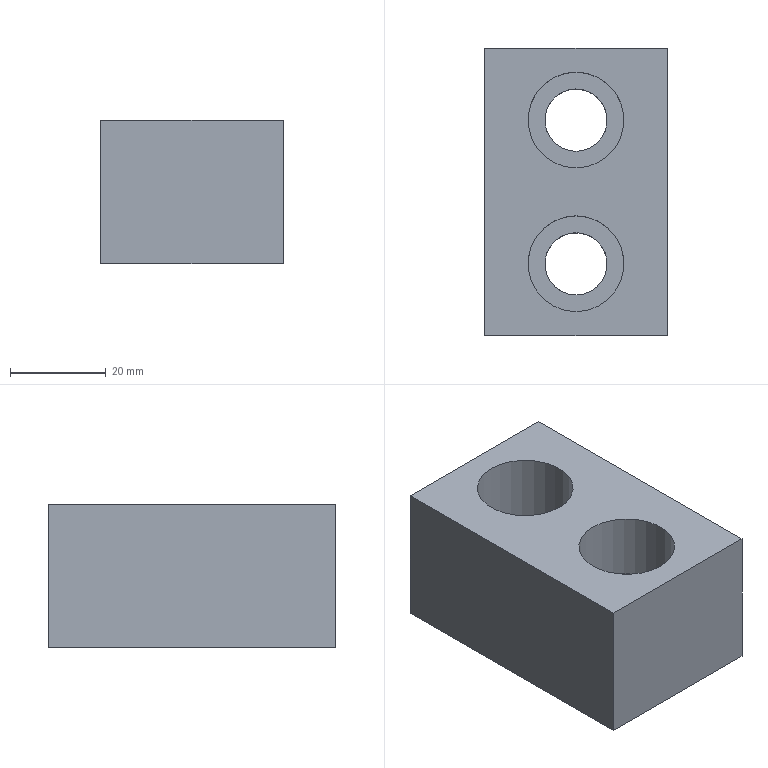Part | NX | features solid 2 | 1 solid | 12 faces | box 38 x 60 x 30 mm | volume 55356 mm3 | plane 8 | cylinder 4 | commonest cylinder face diameters 13 x2 20 x2
STEP:
#1=CARTESIAN_POINT('',(-979.701,85.8,167.));
#2=VERTEX_POINT('',#1);
#3=CARTESIAN_POINT('',(-1017.701,85.8,167.));
#4=VERTEX_POINT('',#3);
#5=CARTESIAN_POINT('',(-979.701,85.8,167.));
#6=DIRECTION('',(-1.,0.,0.));
#7=VECTOR('',#6,1000.);
#8=LINE('',#5,#7);
#9=EDGE_CURVE('',#2,#4,#8,.T.);
#10=ORIENTED_EDGE('',*,*,#9,.F.);
#11=CARTESIAN_POINT('',(-979.701,85.8,197.));
#12=VERTEX_POINT('',#11);
#13=CARTESIAN_POINT('',(-979.701,85.8,187.));
#14=DIRECTION('',(0.,0.,-1.));
#15=VECTOR('',#14,1000.);
#16=LINE('',#13,#15);
#17=EDGE_CURVE('',#12,#2,#16,.T.);
#18=ORIENTED_EDGE('',*,*,#17,.F.);
#19=CARTESIAN_POINT('',(-1017.701,85.8,197.));
#20=VERTEX_POINT('',#19);
#21=CARTESIAN_POINT('',(-979.701,85.8,197.));
#22=DIRECTION('',(-1.,0.,0.));
#23=VECTOR('',#22,1000.);
#24=LINE('',#21,#23);
#25=EDGE_CURVE('',#12,#20,#24,.T.);
#26=ORIENTED_EDGE('',*,*,#25,.T.);
#27=CARTESIAN_POINT('',(-1017.701,85.8,187.));
#28=DIRECTION('',(0.,0.,-1.));
#29=VECTOR('',#28,1000.);
#30=LINE('',#27,#29);
#31=EDGE_CURVE('',#20,#4,#30,.T.);
#32=ORIENTED_EDGE('',*,*,#31,.T.);
#33=EDGE_LOOP('',(#10,#18,#26,#32));
#34=FACE_BOUND('',#33,.T.);
#35=CARTESIAN_POINT('',(-979.701,85.8,187.));
#36=DIRECTION('',(0.,-1.,0.));
#37=DIRECTION('',(1.,0.,0.));
#38=AXIS2_PLACEMENT_3D('',#35,#36,#37);
#39=PLANE('',#38);
#40=ADVANCED_FACE('',(#34),#39,.T.);
#41=CARTESIAN_POINT('',(-1017.701,145.8,167.));
#42=VERTEX_POINT('',#41);
#43=CARTESIAN_POINT('',(-1017.701,85.8,167.));
#44=DIRECTION('',(0.,1.,0.));
#45=VECTOR('',#44,1000.);
#46=LINE('',#43,#45);
#47=EDGE_CURVE('',#4,#42,#46,.T.);
#48=ORIENTED_EDGE('',*,*,#47,.F.);
#49=ORIENTED_EDGE('',*,*,#31,.F.);
#50=CARTESIAN_POINT('',(-1017.701,145.8,197.));
#51=VERTEX_POINT('',#50);
#52=CARTESIAN_POINT('',(-1017.701,85.8,197.));
#53=DIRECTION('',(0.,1.,0.));
#54=VECTOR('',#53,1000.);
#55=LINE('',#52,#54);
#56=EDGE_CURVE('',#20,#51,#55,.T.);
#57=ORIENTED_EDGE('',*,*,#56,.T.);
#58=CARTESIAN_POINT('',(-1017.701,145.8,187.));
#59=DIRECTION('',(0.,0.,-1.));
#60=VECTOR('',#59,1000.);
#61=LINE('',#58,#60);
#62=EDGE_CURVE('',#51,#42,#61,.T.);
#63=ORIENTED_EDGE('',*,*,#62,.T.);
#64=EDGE_LOOP('',(#48,#49,#57,#63));
#65=FACE_BOUND('',#64,.T.);
#66=CARTESIAN_POINT('',(-1017.701,85.8,187.));
#67=DIRECTION('',(-1.,0.,0.));
#68=DIRECTION('',(0.,-1.,0.));
#69=AXIS2_PLACEMENT_3D('',#66,#67,#68);
#70=PLANE('',#69);
#71=ADVANCED_FACE('',(#65),#70,.T.);
#72=CARTESIAN_POINT('',(-979.701,145.8,167.));
#73=VERTEX_POINT('',#72);
#74=CARTESIAN_POINT('',(-1017.701,145.8,167.));
#75=DIRECTION('',(1.,0.,0.));
#76=VECTOR('',#75,1000.);
#77=LINE('',#74,#76);
#78=EDGE_CURVE('',#42,#73,#77,.T.);
#79=ORIENTED_EDGE('',*,*,#78,.F.);
#80=ORIENTED_EDGE('',*,*,#62,.F.);
#81=CARTESIAN_POINT('',(-979.701,145.8,197.));
#82=VERTEX_POINT('',#81);
#83=CARTESIAN_POINT('',(-1017.701,145.8,197.));
#84=DIRECTION('',(1.,0.,0.));
#85=VECTOR('',#84,1000.);
#86=LINE('',#83,#85);
#87=EDGE_CURVE('',#51,#82,#86,.T.);
#88=ORIENTED_EDGE('',*,*,#87,.T.);
#89=CARTESIAN_POINT('',(-979.701,145.8,187.));
#90=DIRECTION('',(0.,0.,-1.));
#91=VECTOR('',#90,1000.);
#92=LINE('',#89,#91);
#93=EDGE_CURVE('',#82,#73,#92,.T.);
#94=ORIENTED_EDGE('',*,*,#93,.T.);
#95=EDGE_LOOP('',(#79,#80,#88,#94));
#96=FACE_BOUND('',#95,.T.);
#97=CARTESIAN_POINT('',(-1017.701,145.8,187.));
#98=DIRECTION('',(0.,1.,0.));
#99=DIRECTION('',(0.,0.,1.));
#100=AXIS2_PLACEMENT_3D('',#97,#98,#99);
#101=PLANE('',#100);
#102=ADVANCED_FACE('',(#96),#101,.T.);
#103=CARTESIAN_POINT('',(-979.701,145.8,167.));
#104=DIRECTION('',(0.,-1.,0.));
#105=VECTOR('',#104,1000.);
#106=LINE('',#103,#105);
#107=EDGE_CURVE('',#73,#2,#106,.T.);
#108=ORIENTED_EDGE('',*,*,#107,.F.);
#109=ORIENTED_EDGE('',*,*,#93,.F.);
#110=CARTESIAN_POINT('',(-979.701,145.8,197.));
#111=DIRECTION('',(0.,-1.,0.));
#112=VECTOR('',#111,1000.);
#113=LINE('',#110,#112);
#114=EDGE_CURVE('',#82,#12,#113,.T.);
#115=ORIENTED_EDGE('',*,*,#114,.T.);
#116=ORIENTED_EDGE('',*,*,#17,.T.);
#117=EDGE_LOOP('',(#108,#109,#115,#116));
#118=FACE_BOUND('',#117,.T.);
#119=CARTESIAN_POINT('',(-979.701,145.8,187.));
#120=DIRECTION('',(1.,0.,0.));
#121=DIRECTION('',(0.,1.,0.));
#122=AXIS2_PLACEMENT_3D('',#119,#120,#121);
#123=PLANE('',#122);
#124=ADVANCED_FACE('',(#118),#123,.T.);
#125=CARTESIAN_POINT('',(-998.701,140.8,197.));
#126=VERTEX_POINT('',#125);
#127=CARTESIAN_POINT('',(-998.701,130.8,197.));
#128=DIRECTION('',(0.,0.,1.));
#129=DIRECTION('',(0.,1.,0.));
#130=AXIS2_PLACEMENT_3D('',#127,#128,#129);
#131=CIRCLE('',#130,10.);
#132=EDGE_CURVE('',#126,#126,#131,.F.);
#133=ORIENTED_EDGE('',*,*,#132,.T.);
#134=EDGE_LOOP('',(#133));
#135=FACE_BOUND('',#134,.T.);
#136=CARTESIAN_POINT('',(-998.701,110.8,197.));
#137=VERTEX_POINT('',#136);
#138=CARTESIAN_POINT('',(-998.701,100.8,197.));
#139=DIRECTION('',(0.,0.,1.));
#140=DIRECTION('',(0.,1.,0.));
#141=AXIS2_PLACEMENT_3D('',#138,#139,#140);
#142=CIRCLE('',#141,10.);
#143=EDGE_CURVE('',#137,#137,#142,.F.);
#144=ORIENTED_EDGE('',*,*,#143,.T.);
#145=EDGE_LOOP('',(#144));
#146=FACE_BOUND('',#145,.T.);
#147=ORIENTED_EDGE('',*,*,#25,.F.);
#148=ORIENTED_EDGE('',*,*,#114,.F.);
#149=ORIENTED_EDGE('',*,*,#87,.F.);
#150=ORIENTED_EDGE('',*,*,#56,.F.);
#151=EDGE_LOOP('',(#147,#148,#149,#150));
#152=FACE_BOUND('',#151,.T.);
#153=CARTESIAN_POINT('',(-979.701,85.8,197.));
#154=DIRECTION('',(0.,0.,1.));
#155=DIRECTION('',(1.,0.,0.));
#156=AXIS2_PLACEMENT_3D('',#153,#154,#155);
#157=PLANE('',#156);
#158=ADVANCED_FACE('',(#135,#146,#152),#157,.T.);
#159=CARTESIAN_POINT('',(-992.201,130.8,167.));
#160=VERTEX_POINT('',#159);
#161=CARTESIAN_POINT('',(-998.701,130.8,167.));
#162=DIRECTION('',(0.,0.,1.));
#163=DIRECTION('',(1.,0.,0.));
#164=AXIS2_PLACEMENT_3D('',#161,#162,#163);
#165=CIRCLE('',#164,6.5);
#166=EDGE_CURVE('',#160,#160,#165,.T.);
#167=ORIENTED_EDGE('',*,*,#166,.T.);
#168=EDGE_LOOP('',(#167));
#169=FACE_BOUND('',#168,.T.);
#170=CARTESIAN_POINT('',(-992.201,100.8,167.));
#171=VERTEX_POINT('',#170);
#172=CARTESIAN_POINT('',(-998.701,100.8,167.));
#173=DIRECTION('',(0.,0.,1.));
#174=DIRECTION('',(1.,0.,0.));
#175=AXIS2_PLACEMENT_3D('',#172,#173,#174);
#176=CIRCLE('',#175,6.5);
#177=EDGE_CURVE('',#171,#171,#176,.T.);
#178=ORIENTED_EDGE('',*,*,#177,.T.);
#179=EDGE_LOOP('',(#178));
#180=FACE_BOUND('',#179,.T.);
#181=ORIENTED_EDGE('',*,*,#9,.T.);
#182=ORIENTED_EDGE('',*,*,#47,.T.);
#183=ORIENTED_EDGE('',*,*,#78,.T.);
#184=ORIENTED_EDGE('',*,*,#107,.T.);
#185=EDGE_LOOP('',(#181,#182,#183,#184));
#186=FACE_BOUND('',#185,.T.);
#187=CARTESIAN_POINT('',(-979.701,85.8,167.));
#188=DIRECTION('',(0.,0.,1.));
#189=DIRECTION('',(1.,0.,0.));
#190=AXIS2_PLACEMENT_3D('',#187,#188,#189);
#191=PLANE('',#190);
#192=ADVANCED_FACE('',(#169,#180,#186),#191,.F.);
#193=CARTESIAN_POINT('',(-998.701,94.3,183.));
#194=VERTEX_POINT('',#193);
#195=CARTESIAN_POINT('',(-998.701,100.8,183.));
#196=DIRECTION('',(0.,0.,-1.));
#197=DIRECTION('',(0.,-1.,0.));
#198=AXIS2_PLACEMENT_3D('',#195,#196,#197);
#199=CIRCLE('',#198,6.5);
#200=EDGE_CURVE('',#194,#194,#199,.T.);
#201=ORIENTED_EDGE('',*,*,#200,.F.);
#202=EDGE_LOOP('',(#201));
#203=FACE_BOUND('',#202,.T.);
#204=ORIENTED_EDGE('',*,*,#177,.F.);
#205=EDGE_LOOP('',(#204));
#206=FACE_BOUND('',#205,.T.);
#207=CARTESIAN_POINT('',(-998.701,100.8,87.));
#208=DIRECTION('',(0.,0.,-1.));
#209=DIRECTION('',(-1.,0.,0.));
#210=AXIS2_PLACEMENT_3D('',#207,#208,#209);
#211=CYLINDRICAL_SURFACE('',#210,6.5);
#212=ADVANCED_FACE('',(#203,#206),#211,.F.);
#213=ORIENTED_EDGE('',*,*,#200,.T.);
#214=EDGE_LOOP('',(#213));
#215=FACE_BOUND('',#214,.T.);
#216=CARTESIAN_POINT('',(-998.701,90.8,183.));
#217=VERTEX_POINT('',#216);
#218=CARTESIAN_POINT('',(-998.701,100.8,183.));
#219=DIRECTION('',(0.,0.,-1.));
#220=DIRECTION('',(0.,-1.,0.));
#221=AXIS2_PLACEMENT_3D('',#218,#219,#220);
#222=CIRCLE('',#221,10.);
#223=EDGE_CURVE('',#217,#217,#222,.T.);
#224=ORIENTED_EDGE('',*,*,#223,.F.);
#225=EDGE_LOOP('',(#224));
#226=FACE_BOUND('',#225,.T.);
#227=CARTESIAN_POINT('',(-998.701,100.8,183.));
#228=DIRECTION('',(0.,0.,-1.));
#229=DIRECTION('',(-1.,0.,0.));
#230=AXIS2_PLACEMENT_3D('',#227,#228,#229);
#231=PLANE('',#230);
#232=ADVANCED_FACE('',(#215,#226),#231,.F.);
#233=ORIENTED_EDGE('',*,*,#223,.T.);
#234=EDGE_LOOP('',(#233));
#235=FACE_BOUND('',#234,.T.);
#236=ORIENTED_EDGE('',*,*,#143,.F.);
#237=EDGE_LOOP('',(#236));
#238=FACE_BOUND('',#237,.T.);
#239=CARTESIAN_POINT('',(-998.701,100.8,187.));
#240=DIRECTION('',(0.,0.,-1.));
#241=DIRECTION('',(-1.,0.,0.));
#242=AXIS2_PLACEMENT_3D('',#239,#240,#241);
#243=CYLINDRICAL_SURFACE('',#242,10.);
#244=ADVANCED_FACE('',(#235,#238),#243,.F.);
#245=CARTESIAN_POINT('',(-998.701,124.3,183.));
#246=VERTEX_POINT('',#245);
#247=CARTESIAN_POINT('',(-998.701,130.8,183.));
#248=DIRECTION('',(0.,0.,-1.));
#249=DIRECTION('',(0.,-1.,0.));
#250=AXIS2_PLACEMENT_3D('',#247,#248,#249);
#251=CIRCLE('',#250,6.5);
#252=EDGE_CURVE('',#246,#246,#251,.T.);
#253=ORIENTED_EDGE('',*,*,#252,.F.);
#254=EDGE_LOOP('',(#253));
#255=FACE_BOUND('',#254,.T.);
#256=ORIENTED_EDGE('',*,*,#166,.F.);
#257=EDGE_LOOP('',(#256));
#258=FACE_BOUND('',#257,.T.);
#259=CARTESIAN_POINT('',(-998.701,130.8,87.));
#260=DIRECTION('',(0.,0.,-1.));
#261=DIRECTION('',(-1.,0.,0.));
#262=AXIS2_PLACEMENT_3D('',#259,#260,#261);
#263=CYLINDRICAL_SURFACE('',#262,6.5);
#264=ADVANCED_FACE('',(#255,#258),#263,.F.);
#265=ORIENTED_EDGE('',*,*,#252,.T.);
#266=EDGE_LOOP('',(#265));
#267=FACE_BOUND('',#266,.T.);
#268=CARTESIAN_POINT('',(-998.701,120.8,183.));
#269=VERTEX_POINT('',#268);
#270=CARTESIAN_POINT('',(-998.701,130.8,183.));
#271=DIRECTION('',(0.,0.,-1.));
#272=DIRECTION('',(0.,-1.,0.));
#273=AXIS2_PLACEMENT_3D('',#270,#271,#272);
#274=CIRCLE('',#273,10.);
#275=EDGE_CURVE('',#269,#269,#274,.T.);
#276=ORIENTED_EDGE('',*,*,#275,.F.);
#277=EDGE_LOOP('',(#276));
#278=FACE_BOUND('',#277,.T.);
#279=CARTESIAN_POINT('',(-998.701,130.8,183.));
#280=DIRECTION('',(0.,0.,-1.));
#281=DIRECTION('',(-1.,0.,0.));
#282=AXIS2_PLACEMENT_3D('',#279,#280,#281);
#283=PLANE('',#282);
#284=ADVANCED_FACE('',(#267,#278),#283,.F.);
#285=ORIENTED_EDGE('',*,*,#275,.T.);
#286=EDGE_LOOP('',(#285));
#287=FACE_BOUND('',#286,.T.);
#288=ORIENTED_EDGE('',*,*,#132,.F.);
#289=EDGE_LOOP('',(#288));
#290=FACE_BOUND('',#289,.T.);
#291=CARTESIAN_POINT('',(-998.701,130.8,187.));
#292=DIRECTION('',(0.,0.,-1.));
#293=DIRECTION('',(-1.,0.,0.));
#294=AXIS2_PLACEMENT_3D('',#291,#292,#293);
#295=CYLINDRICAL_SURFACE('',#294,10.);
#296=ADVANCED_FACE('',(#287,#290),#295,.F.);
#297=CLOSED_SHELL('',(#40,#71,#102,#124,#158,#192,#212,#232,#244,#264,#284,#296));
#298=MANIFOLD_SOLID_BREP('',#297);
#299=(LENGTH_UNIT()NAMED_UNIT(*)SI_UNIT(.MILLI.,.METRE.));
#300=UNCERTAINTY_MEASURE_WITH_UNIT(LENGTH_MEASURE(0.00001),#299,'','');
#301=(NAMED_UNIT(*)PLANE_ANGLE_UNIT()SI_UNIT($,.RADIAN.));
#302=(NAMED_UNIT(*)SI_UNIT($,.STERADIAN.)SOLID_ANGLE_UNIT());
#303=(GEOMETRIC_REPRESENTATION_CONTEXT(3)GLOBAL_UNCERTAINTY_ASSIGNED_CONTEXT((#300))GLOBAL_UNIT_ASSIGNED_CONTEXT((#299,#301,#302))REPRESENTATION_CONTEXT('',''));
#304=ADVANCED_BREP_SHAPE_REPRESENTATION('',(#298),#303);